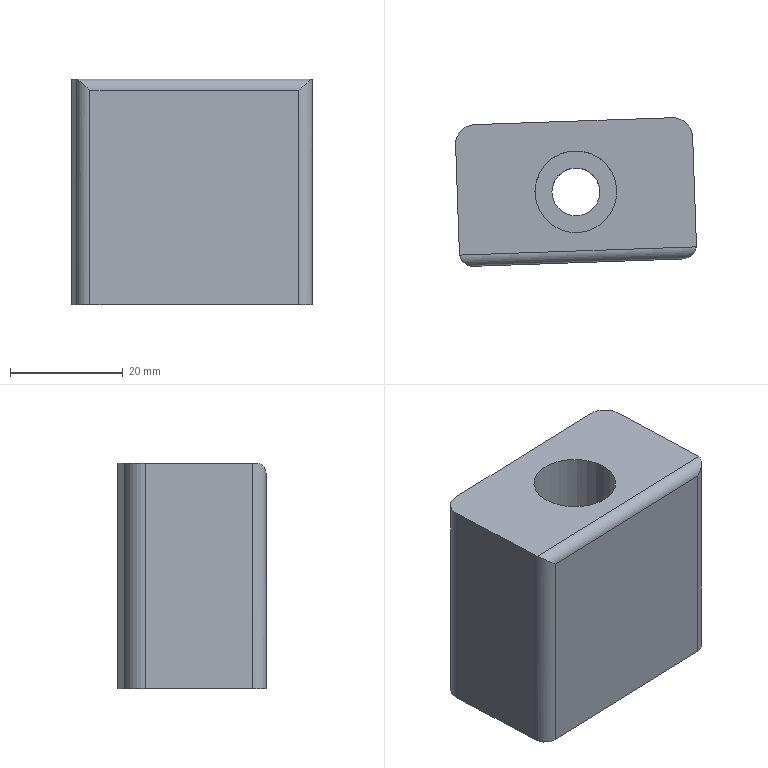Part | NX | features DIE-67 2 | 1 solid | 14 faces | box 42.641 x 26.245 x 40 mm | volume 37753 mm3 | plane 7 | cylinder 7 | commonest cylinder face diameters 5 x2 7 x2 4 x1 8.5 x1 14.5 x1
STEP:
#1=CARTESIAN_POINT('',(3516.285,-779.688,823.716));
#2=VERTEX_POINT('',#1);
#3=CARTESIAN_POINT('',(3512.035,-779.688,823.716));
#4=DIRECTION('',(0.,0.,1.));
#5=DIRECTION('',(1.,0.,0.));
#6=AXIS2_PLACEMENT_3D('',#3,#4,#5);
#7=CIRCLE('',#6,4.25);
#8=EDGE_CURVE('',#2,#2,#7,.T.);
#9=ORIENTED_EDGE('',*,*,#8,.T.);
#10=EDGE_LOOP('',(#9));
#11=FACE_BOUND('',#10,.T.);
#12=CARTESIAN_POINT('',(3494.11,-767.806,823.716));
#13=VERTEX_POINT('',#12);
#14=CARTESIAN_POINT('',(3529.089,-766.585,823.716));
#15=VERTEX_POINT('',#14);
#16=CARTESIAN_POINT('',(3525.325,-766.717,823.716));
#17=DIRECTION('',(0.9994,0.0349,0.));
#18=VECTOR('',#17,1000.);
#19=LINE('',#16,#18);
#20=EDGE_CURVE('',#13,#15,#19,.T.);
#21=ORIENTED_EDGE('',*,*,#20,.T.);
#22=CARTESIAN_POINT('',(3532.709,-769.961,823.716));
#23=VERTEX_POINT('',#22);
#24=CARTESIAN_POINT('',(3529.211,-770.083,823.716));
#25=DIRECTION('',(0.,0.,1.));
#26=DIRECTION('',(1.,0.,0.));
#27=AXIS2_PLACEMENT_3D('',#24,#25,#26);
#28=CIRCLE('',#27,3.5);
#29=EDGE_CURVE('',#15,#23,#28,.F.);
#30=ORIENTED_EDGE('',*,*,#29,.T.);
#31=CARTESIAN_POINT('',(3533.372,-788.949,823.716));
#32=VERTEX_POINT('',#31);
#33=CARTESIAN_POINT('',(3535.133,-839.387,823.716));
#34=DIRECTION('',(0.0349,-0.9994,0.));
#35=VECTOR('',#34,1000.);
#36=LINE('',#33,#35);
#37=EDGE_CURVE('',#23,#32,#36,.T.);
#38=ORIENTED_EDGE('',*,*,#37,.T.);
#39=CARTESIAN_POINT('',(3530.96,-791.535,823.716));
#40=VERTEX_POINT('',#39);
#41=CARTESIAN_POINT('',(3530.873,-789.037,823.716));
#42=DIRECTION('',(0.,0.,1.));
#43=DIRECTION('',(1.,0.,0.));
#44=AXIS2_PLACEMENT_3D('',#41,#42,#43);
#45=CIRCLE('',#44,2.5);
#46=EDGE_CURVE('',#32,#40,#45,.F.);
#47=ORIENTED_EDGE('',*,*,#46,.T.);
#48=CARTESIAN_POINT('',(3493.983,-792.826,823.716));
#49=VERTEX_POINT('',#48);
#50=CARTESIAN_POINT('',(3526.198,-791.701,823.716));
#51=DIRECTION('',(0.9994,0.0349,0.));
#52=VECTOR('',#51,1000.);
#53=LINE('',#50,#52);
#54=EDGE_CURVE('',#49,#40,#53,.T.);
#55=ORIENTED_EDGE('',*,*,#54,.F.);
#56=CARTESIAN_POINT('',(3491.397,-790.415,823.716));
#57=VERTEX_POINT('',#56);
#58=CARTESIAN_POINT('',(3493.896,-790.328,823.716));
#59=DIRECTION('',(0.,0.,1.));
#60=DIRECTION('',(1.,0.,0.));
#61=AXIS2_PLACEMENT_3D('',#58,#59,#60);
#62=CIRCLE('',#61,2.5);
#63=EDGE_CURVE('',#49,#57,#62,.F.);
#64=ORIENTED_EDGE('',*,*,#63,.T.);
#65=CARTESIAN_POINT('',(3490.734,-771.426,823.716));
#66=VERTEX_POINT('',#65);
#67=CARTESIAN_POINT('',(3492.21,-813.679,823.716));
#68=DIRECTION('',(-0.0349,0.9994,0.));
#69=VECTOR('',#68,1000.);
#70=LINE('',#67,#69);
#71=EDGE_CURVE('',#66,#57,#70,.F.);
#72=ORIENTED_EDGE('',*,*,#71,.F.);
#73=CARTESIAN_POINT('',(3494.232,-771.304,823.716));
#74=DIRECTION('',(0.,0.,1.));
#75=DIRECTION('',(1.,0.,0.));
#76=AXIS2_PLACEMENT_3D('',#73,#74,#75);
#77=CIRCLE('',#76,3.5);
#78=EDGE_CURVE('',#66,#13,#77,.F.);
#79=ORIENTED_EDGE('',*,*,#78,.T.);
#80=EDGE_LOOP('',(#21,#30,#38,#47,#55,#64,#72,#79));
#81=FACE_BOUND('',#80,.T.);
#82=CARTESIAN_POINT('',(3542.707,-839.123,823.716));
#83=DIRECTION('',(0.,0.,1.));
#84=DIRECTION('',(0.,-1.,0.));
#85=AXIS2_PLACEMENT_3D('',#82,#83,#84);
#86=PLANE('',#85);
#87=ADVANCED_FACE('',(#11,#81),#86,.F.);
#88=ORIENTED_EDGE('',*,*,#37,.F.);
#89=CARTESIAN_POINT('',(3532.709,-769.961,863.716));
#90=VERTEX_POINT('',#89);
#91=CARTESIAN_POINT('',(3532.709,-769.961,863.716));
#92=DIRECTION('',(0.,0.,-1.));
#93=VECTOR('',#92,1000.);
#94=LINE('',#91,#93);
#95=EDGE_CURVE('',#23,#90,#94,.F.);
#96=ORIENTED_EDGE('',*,*,#95,.T.);
#97=CARTESIAN_POINT('',(3533.372,-788.949,863.716));
#98=VERTEX_POINT('',#97);
#99=CARTESIAN_POINT('',(3533.977,-806.297,863.716));
#100=DIRECTION('',(-0.0349,0.9994,0.));
#101=VECTOR('',#100,1000.);
#102=LINE('',#99,#101);
#103=EDGE_CURVE('',#90,#98,#102,.F.);
#104=ORIENTED_EDGE('',*,*,#103,.T.);
#105=CARTESIAN_POINT('',(3533.372,-788.949,891.507));
#106=DIRECTION('',(0.,0.,1.));
#107=VECTOR('',#106,1000.);
#108=LINE('',#105,#107);
#109=EDGE_CURVE('',#98,#32,#108,.F.);
#110=ORIENTED_EDGE('',*,*,#109,.T.);
#111=EDGE_LOOP('',(#88,#96,#104,#110));
#112=FACE_BOUND('',#111,.T.);
#113=CARTESIAN_POINT('',(3533.977,-806.297,891.507));
#114=DIRECTION('',(-0.9994,-0.0349,0.));
#115=DIRECTION('',(-0.0349,0.9994,0.));
#116=AXIS2_PLACEMENT_3D('',#113,#114,#115);
#117=PLANE('',#116);
#118=ADVANCED_FACE('',(#112),#117,.F.);
#119=CARTESIAN_POINT('',(3519.285,-779.688,863.716));
#120=VERTEX_POINT('',#119);
#121=CARTESIAN_POINT('',(3512.035,-779.688,863.716));
#122=DIRECTION('',(0.,0.,1.));
#123=DIRECTION('',(1.,0.,0.));
#124=AXIS2_PLACEMENT_3D('',#121,#122,#123);
#125=CIRCLE('',#124,7.25);
#126=EDGE_CURVE('',#120,#120,#125,.F.);
#127=ORIENTED_EDGE('',*,*,#126,.T.);
#128=EDGE_LOOP('',(#127));
#129=FACE_BOUND('',#128,.T.);
#130=ORIENTED_EDGE('',*,*,#103,.F.);
#131=CARTESIAN_POINT('',(3529.089,-766.585,863.716));
#132=VERTEX_POINT('',#131);
#133=CARTESIAN_POINT('',(3529.211,-770.083,863.716));
#134=DIRECTION('',(0.,0.,1.));
#135=DIRECTION('',(1.,0.,0.));
#136=AXIS2_PLACEMENT_3D('',#133,#134,#135);
#137=CIRCLE('',#136,3.5);
#138=EDGE_CURVE('',#90,#132,#137,.T.);
#139=ORIENTED_EDGE('',*,*,#138,.T.);
#140=CARTESIAN_POINT('',(3494.11,-767.806,863.716));
#141=VERTEX_POINT('',#140);
#142=CARTESIAN_POINT('',(3525.325,-766.717,863.716));
#143=DIRECTION('',(0.9994,0.0349,0.));
#144=VECTOR('',#143,1000.);
#145=LINE('',#142,#144);
#146=EDGE_CURVE('',#132,#141,#145,.F.);
#147=ORIENTED_EDGE('',*,*,#146,.T.);
#148=CARTESIAN_POINT('',(3490.734,-771.426,863.716));
#149=VERTEX_POINT('',#148);
#150=CARTESIAN_POINT('',(3494.232,-771.304,863.716));
#151=DIRECTION('',(0.,0.,1.));
#152=DIRECTION('',(1.,0.,0.));
#153=AXIS2_PLACEMENT_3D('',#150,#151,#152);
#154=CIRCLE('',#153,3.5);
#155=EDGE_CURVE('',#141,#149,#154,.T.);
#156=ORIENTED_EDGE('',*,*,#155,.T.);
#157=CARTESIAN_POINT('',(3491.397,-790.415,863.716));
#158=VERTEX_POINT('',#157);
#159=CARTESIAN_POINT('',(3493.158,-840.853,863.716));
#160=DIRECTION('',(0.0349,-0.9994,0.));
#161=VECTOR('',#160,1000.);
#162=LINE('',#159,#161);
#163=EDGE_CURVE('',#149,#158,#162,.T.);
#164=ORIENTED_EDGE('',*,*,#163,.T.);
#165=CARTESIAN_POINT('',(3491.465,-790.913,863.716));
#166=VERTEX_POINT('',#165);
#167=CARTESIAN_POINT('',(3493.896,-790.328,863.716));
#168=DIRECTION('',(0.,0.,1.));
#169=DIRECTION('',(1.,0.,0.));
#170=AXIS2_PLACEMENT_3D('',#167,#168,#169);
#171=CIRCLE('',#170,2.5);
#172=EDGE_CURVE('',#158,#166,#171,.T.);
#173=ORIENTED_EDGE('',*,*,#172,.T.);
#174=CARTESIAN_POINT('',(3533.339,-789.451,863.716));
#175=VERTEX_POINT('',#174);
#176=CARTESIAN_POINT('',(3540.963,-789.185,863.716));
#177=DIRECTION('',(-0.9994,-0.0349,0.));
#178=VECTOR('',#177,1000.);
#179=LINE('',#176,#178);
#180=EDGE_CURVE('',#175,#166,#179,.T.);
#181=ORIENTED_EDGE('',*,*,#180,.F.);
#182=CARTESIAN_POINT('',(3530.873,-789.037,863.716));
#183=DIRECTION('',(0.,0.,1.));
#184=DIRECTION('',(1.,0.,0.));
#185=AXIS2_PLACEMENT_3D('',#182,#183,#184);
#186=CIRCLE('',#185,2.5);
#187=EDGE_CURVE('',#175,#98,#186,.T.);
#188=ORIENTED_EDGE('',*,*,#187,.T.);
#189=EDGE_LOOP('',(#130,#139,#147,#156,#164,#173,#181,#188));
#190=FACE_BOUND('',#189,.T.);
#191=CARTESIAN_POINT('',(3542.707,-839.123,863.716));
#192=DIRECTION('',(0.,0.,1.));
#193=DIRECTION('',(0.,-1.,0.));
#194=AXIS2_PLACEMENT_3D('',#191,#192,#193);
#195=PLANE('',#194);
#196=ADVANCED_FACE('',(#129,#190),#195,.T.);
#197=ORIENTED_EDGE('',*,*,#163,.F.);
#198=CARTESIAN_POINT('',(3490.734,-771.426,823.716));
#199=DIRECTION('',(0.,0.,1.));
#200=VECTOR('',#199,1000.);
#201=LINE('',#198,#200);
#202=EDGE_CURVE('',#149,#66,#201,.F.);
#203=ORIENTED_EDGE('',*,*,#202,.T.);
#204=ORIENTED_EDGE('',*,*,#71,.T.);
#205=CARTESIAN_POINT('',(3491.397,-790.415,948.075));
#206=DIRECTION('',(0.,0.,1.));
#207=VECTOR('',#206,1000.);
#208=LINE('',#205,#207);
#209=EDGE_CURVE('',#57,#158,#208,.T.);
#210=ORIENTED_EDGE('',*,*,#209,.T.);
#211=EDGE_LOOP('',(#197,#203,#204,#210));
#212=FACE_BOUND('',#211,.T.);
#213=CARTESIAN_POINT('',(3492.21,-813.679,948.075));
#214=DIRECTION('',(-0.9994,-0.0349,0.));
#215=DIRECTION('',(-0.0349,0.9994,0.));
#216=AXIS2_PLACEMENT_3D('',#213,#214,#215);
#217=PLANE('',#216);
#218=ADVANCED_FACE('',(#212),#217,.T.);
#219=ORIENTED_EDGE('',*,*,#146,.F.);
#220=CARTESIAN_POINT('',(3529.089,-766.585,823.716));
#221=DIRECTION('',(0.,0.,-1.));
#222=VECTOR('',#221,1000.);
#223=LINE('',#220,#222);
#224=EDGE_CURVE('',#132,#15,#223,.T.);
#225=ORIENTED_EDGE('',*,*,#224,.T.);
#226=ORIENTED_EDGE('',*,*,#20,.F.);
#227=CARTESIAN_POINT('',(3494.11,-767.806,863.716));
#228=DIRECTION('',(0.,0.,-1.));
#229=VECTOR('',#228,1000.);
#230=LINE('',#227,#229);
#231=EDGE_CURVE('',#13,#141,#230,.F.);
#232=ORIENTED_EDGE('',*,*,#231,.T.);
#233=EDGE_LOOP('',(#219,#225,#226,#232));
#234=FACE_BOUND('',#233,.T.);
#235=CARTESIAN_POINT('',(3525.325,-766.717,940.297));
#236=DIRECTION('',(-0.0349,0.9994,0.));
#237=DIRECTION('',(0.9994,0.0349,0.));
#238=AXIS2_PLACEMENT_3D('',#235,#236,#237);
#239=PLANE('',#238);
#240=ADVANCED_FACE('',(#234),#239,.T.);
#241=ORIENTED_EDGE('',*,*,#54,.T.);
#242=CARTESIAN_POINT('',(3530.96,-791.535,861.716));
#243=VERTEX_POINT('',#242);
#244=CARTESIAN_POINT('',(3530.96,-791.535,940.297));
#245=DIRECTION('',(0.,0.,1.));
#246=VECTOR('',#245,1000.);
#247=LINE('',#244,#246);
#248=EDGE_CURVE('',#40,#243,#247,.T.);
#249=ORIENTED_EDGE('',*,*,#248,.T.);
#250=CARTESIAN_POINT('',(3493.983,-792.826,861.716));
#251=VERTEX_POINT('',#250);
#252=CARTESIAN_POINT('',(3526.198,-791.701,861.716));
#253=DIRECTION('',(0.9994,0.0349,0.));
#254=VECTOR('',#253,1000.);
#255=LINE('',#252,#254);
#256=EDGE_CURVE('',#251,#243,#255,.T.);
#257=ORIENTED_EDGE('',*,*,#256,.F.);
#258=CARTESIAN_POINT('',(3493.983,-792.826,940.297));
#259=DIRECTION('',(0.,0.,-1.));
#260=VECTOR('',#259,1000.);
#261=LINE('',#258,#260);
#262=EDGE_CURVE('',#251,#49,#261,.T.);
#263=ORIENTED_EDGE('',*,*,#262,.T.);
#264=EDGE_LOOP('',(#241,#249,#257,#263));
#265=FACE_BOUND('',#264,.T.);
#266=CARTESIAN_POINT('',(3526.198,-791.701,940.297));
#267=DIRECTION('',(-0.0349,0.9994,0.));
#268=DIRECTION('',(0.9994,0.0349,0.));
#269=AXIS2_PLACEMENT_3D('',#266,#267,#268);
#270=PLANE('',#269);
#271=ADVANCED_FACE('',(#265),#270,.F.);
#272=ORIENTED_EDGE('',*,*,#256,.T.);
#273=CARTESIAN_POINT('',(3533.339,-789.451,863.716));
#274=CARTESIAN_POINT('',(3533.225,-790.126,863.716));
#275=CARTESIAN_POINT('',(3532.462,-791.207,863.069));
#276=CARTESIAN_POINT('',(3531.461,-791.518,862.165));
#277=CARTESIAN_POINT('',(3530.96,-791.535,861.716));
#278=B_SPLINE_CURVE_WITH_KNOTS('',3,(#273,#274,#275,#276,#277),.UNSPECIFIED.,.F.,.F.,(4,1,4),(0.,0.002017,0.004035),.UNSPECIFIED.);
#279=EDGE_CURVE('',#243,#175,#278,.F.);
#280=ORIENTED_EDGE('',*,*,#279,.T.);
#281=ORIENTED_EDGE('',*,*,#180,.T.);
#282=CARTESIAN_POINT('',(3491.465,-790.913,863.716));
#283=CARTESIAN_POINT('',(3491.625,-791.578,863.716));
#284=CARTESIAN_POINT('',(3492.462,-792.603,863.069));
#285=CARTESIAN_POINT('',(3493.482,-792.844,862.165));
#286=CARTESIAN_POINT('',(3493.983,-792.826,861.716));
#287=B_SPLINE_CURVE_WITH_KNOTS('',3,(#282,#283,#284,#285,#286),.UNSPECIFIED.,.F.,.F.,(4,1,4),(0.,0.002017,0.004035),.UNSPECIFIED.);
#288=EDGE_CURVE('',#166,#251,#287,.T.);
#289=ORIENTED_EDGE('',*,*,#288,.T.);
#290=EDGE_LOOP('',(#272,#280,#281,#289));
#291=FACE_BOUND('',#290,.T.);
#292=CARTESIAN_POINT('',(3540.963,-789.185,861.716));
#293=DIRECTION('',(0.9994,0.0349,0.));
#294=DIRECTION('',(0.0349,-0.9994,0.));
#295=AXIS2_PLACEMENT_3D('',#292,#293,#294);
#296=CYLINDRICAL_SURFACE('',#295,2.);
#297=ADVANCED_FACE('',(#291),#296,.T.);
#298=ORIENTED_EDGE('',*,*,#46,.F.);
#299=ORIENTED_EDGE('',*,*,#109,.F.);
#300=ORIENTED_EDGE('',*,*,#187,.F.);
#301=ORIENTED_EDGE('',*,*,#279,.F.);
#302=ORIENTED_EDGE('',*,*,#248,.F.);
#303=EDGE_LOOP('',(#298,#299,#300,#301,#302));
#304=FACE_BOUND('',#303,.T.);
#305=CARTESIAN_POINT('',(3530.873,-789.037,940.297));
#306=DIRECTION('',(0.,0.,1.));
#307=DIRECTION('',(1.,0.,0.));
#308=AXIS2_PLACEMENT_3D('',#305,#306,#307);
#309=CYLINDRICAL_SURFACE('',#308,2.5);
#310=ADVANCED_FACE('',(#304),#309,.T.);
#311=ORIENTED_EDGE('',*,*,#63,.F.);
#312=ORIENTED_EDGE('',*,*,#262,.F.);
#313=ORIENTED_EDGE('',*,*,#288,.F.);
#314=ORIENTED_EDGE('',*,*,#172,.F.);
#315=ORIENTED_EDGE('',*,*,#209,.F.);
#316=EDGE_LOOP('',(#311,#312,#313,#314,#315));
#317=FACE_BOUND('',#316,.T.);
#318=CARTESIAN_POINT('',(3493.896,-790.328,948.075));
#319=DIRECTION('',(0.,0.,-1.));
#320=DIRECTION('',(-1.,0.,0.));
#321=AXIS2_PLACEMENT_3D('',#318,#319,#320);
#322=CYLINDRICAL_SURFACE('',#321,2.5);
#323=ADVANCED_FACE('',(#317),#322,.T.);
#324=ORIENTED_EDGE('',*,*,#138,.F.);
#325=ORIENTED_EDGE('',*,*,#95,.F.);
#326=ORIENTED_EDGE('',*,*,#29,.F.);
#327=ORIENTED_EDGE('',*,*,#224,.F.);
#328=EDGE_LOOP('',(#324,#325,#326,#327));
#329=FACE_BOUND('',#328,.T.);
#330=CARTESIAN_POINT('',(3529.211,-770.083,940.297));
#331=DIRECTION('',(0.,0.,1.));
#332=DIRECTION('',(1.,0.,0.));
#333=AXIS2_PLACEMENT_3D('',#330,#331,#332);
#334=CYLINDRICAL_SURFACE('',#333,3.5);
#335=ADVANCED_FACE('',(#329),#334,.T.);
#336=ORIENTED_EDGE('',*,*,#78,.F.);
#337=ORIENTED_EDGE('',*,*,#202,.F.);
#338=ORIENTED_EDGE('',*,*,#155,.F.);
#339=ORIENTED_EDGE('',*,*,#231,.F.);
#340=EDGE_LOOP('',(#336,#337,#338,#339));
#341=FACE_BOUND('',#340,.T.);
#342=CARTESIAN_POINT('',(3494.232,-771.304,940.297));
#343=DIRECTION('',(0.,0.,1.));
#344=DIRECTION('',(1.,0.,0.));
#345=AXIS2_PLACEMENT_3D('',#342,#343,#344);
#346=CYLINDRICAL_SURFACE('',#345,3.5);
#347=ADVANCED_FACE('',(#341),#346,.T.);
#348=CARTESIAN_POINT('',(3516.285,-779.688,848.716));
#349=VERTEX_POINT('',#348);
#350=CARTESIAN_POINT('',(3512.035,-779.688,848.716));
#351=DIRECTION('',(0.,0.,1.));
#352=DIRECTION('',(1.,0.,0.));
#353=AXIS2_PLACEMENT_3D('',#350,#351,#352);
#354=CIRCLE('',#353,4.25);
#355=EDGE_CURVE('',#349,#349,#354,.T.);
#356=ORIENTED_EDGE('',*,*,#355,.T.);
#357=EDGE_LOOP('',(#356));
#358=FACE_BOUND('',#357,.T.);
#359=ORIENTED_EDGE('',*,*,#8,.F.);
#360=EDGE_LOOP('',(#359));
#361=FACE_BOUND('',#360,.T.);
#362=CARTESIAN_POINT('',(3512.035,-779.688,822.716));
#363=DIRECTION('',(0.,0.,1.));
#364=DIRECTION('',(1.,0.,0.));
#365=AXIS2_PLACEMENT_3D('',#362,#363,#364);
#366=CYLINDRICAL_SURFACE('',#365,4.25);
#367=ADVANCED_FACE('',(#358,#361),#366,.F.);
#368=CARTESIAN_POINT('',(3504.79,-779.941,848.716));
#369=VERTEX_POINT('',#368);
#370=CARTESIAN_POINT('',(3512.035,-779.688,848.716));
#371=DIRECTION('',(0.,0.,1.));
#372=DIRECTION('',(-0.9994,-0.0349,0.));
#373=AXIS2_PLACEMENT_3D('',#370,#371,#372);
#374=CIRCLE('',#373,7.25);
#375=EDGE_CURVE('',#369,#369,#374,.F.);
#376=ORIENTED_EDGE('',*,*,#375,.T.);
#377=EDGE_LOOP('',(#376));
#378=FACE_BOUND('',#377,.T.);
#379=ORIENTED_EDGE('',*,*,#126,.F.);
#380=EDGE_LOOP('',(#379));
#381=FACE_BOUND('',#380,.T.);
#382=CARTESIAN_POINT('',(3512.035,-779.688,848.716));
#383=DIRECTION('',(0.,0.,1.));
#384=DIRECTION('',(1.,0.,0.));
#385=AXIS2_PLACEMENT_3D('',#382,#383,#384);
#386=CYLINDRICAL_SURFACE('',#385,7.25);
#387=ADVANCED_FACE('',(#378,#381),#386,.F.);
#388=ORIENTED_EDGE('',*,*,#355,.F.);
#389=EDGE_LOOP('',(#388));
#390=FACE_BOUND('',#389,.T.);
#391=ORIENTED_EDGE('',*,*,#375,.F.);
#392=EDGE_LOOP('',(#391));
#393=FACE_BOUND('',#392,.T.);
#394=CARTESIAN_POINT('',(3512.035,-779.688,848.716));
#395=DIRECTION('',(0.,0.,1.));
#396=DIRECTION('',(1.,0.,0.));
#397=AXIS2_PLACEMENT_3D('',#394,#395,#396);
#398=PLANE('',#397);
#399=ADVANCED_FACE('',(#390,#393),#398,.T.);
#400=CLOSED_SHELL('',(#87,#118,#196,#218,#240,#271,#297,#310,#323,#335,#347,#367,#387,#399));
#401=MANIFOLD_SOLID_BREP('',#400);
#402=(LENGTH_UNIT()NAMED_UNIT(*)SI_UNIT(.MILLI.,.METRE.));
#403=UNCERTAINTY_MEASURE_WITH_UNIT(LENGTH_MEASURE(0.0508),#402,'','');
#404=(NAMED_UNIT(*)PLANE_ANGLE_UNIT()SI_UNIT($,.RADIAN.));
#405=(NAMED_UNIT(*)SI_UNIT($,.STERADIAN.)SOLID_ANGLE_UNIT());
#406=(GEOMETRIC_REPRESENTATION_CONTEXT(3)GLOBAL_UNCERTAINTY_ASSIGNED_CONTEXT((#403))GLOBAL_UNIT_ASSIGNED_CONTEXT((#402,#404,#405))REPRESENTATION_CONTEXT('',''));
#407=ADVANCED_BREP_SHAPE_REPRESENTATION('',(#401),#406);